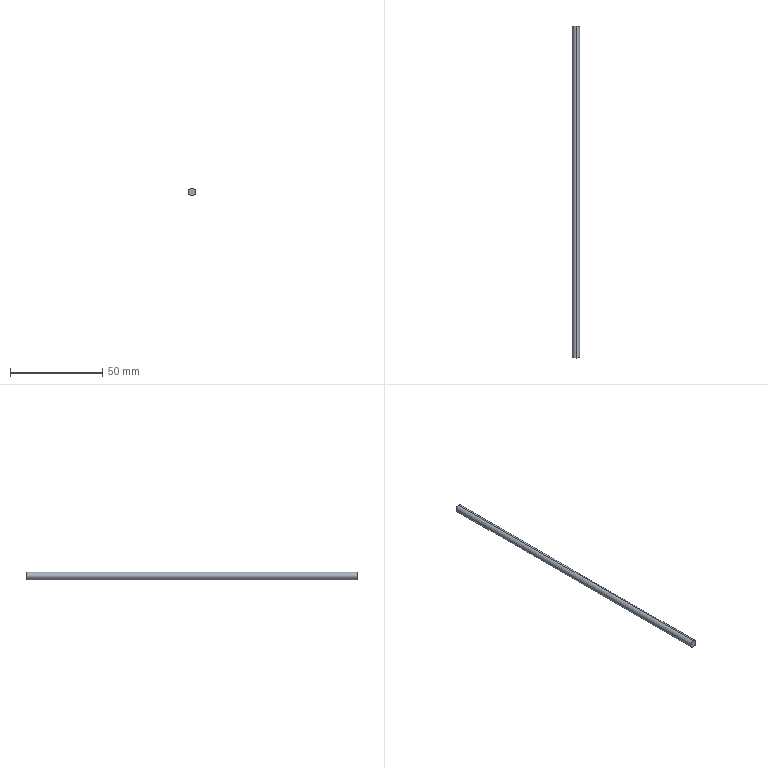Part | SolidWorks | features Extrusion 1 | 1 solid | 4 faces | box 4 x 180 x 4 mm | volume 2262 mm3 | cylinder 2 | plane 2 | commonest cylinder face diameters 4 x2
STEP:
#1=CARTESIAN_POINT('',(0.,180.,2.));
#2=VERTEX_POINT('',#1);
#3=CARTESIAN_POINT('',(0.,180.,-2.));
#4=VERTEX_POINT('',#3);
#5=CARTESIAN_POINT('',(0.,180.,0.));
#6=DIRECTION('',(0.,1.,0.));
#7=DIRECTION('',(0.,0.,1.));
#8=AXIS2_PLACEMENT_3D('',#5,#6,#7);
#9=CIRCLE('',#8,2.);
#10=EDGE_CURVE('',#2,#4,#9,.T.);
#11=ORIENTED_EDGE('',*,*,#10,.F.);
#12=CARTESIAN_POINT('',(0.,0.,2.));
#13=VERTEX_POINT('',#12);
#14=CARTESIAN_POINT('',(0.,180.,2.));
#15=DIRECTION('',(0.,-1.,0.));
#16=VECTOR('',#15,1000.);
#17=LINE('',#14,#16);
#18=EDGE_CURVE('',#2,#13,#17,.T.);
#19=ORIENTED_EDGE('',*,*,#18,.T.);
#20=CARTESIAN_POINT('',(0.,0.,-2.));
#21=VERTEX_POINT('',#20);
#22=CARTESIAN_POINT('',(0.,0.,0.));
#23=DIRECTION('',(0.,1.,0.));
#24=DIRECTION('',(0.,0.,1.));
#25=AXIS2_PLACEMENT_3D('',#22,#23,#24);
#26=CIRCLE('',#25,2.);
#27=EDGE_CURVE('',#13,#21,#26,.T.);
#28=ORIENTED_EDGE('',*,*,#27,.T.);
#29=CARTESIAN_POINT('',(0.,180.,-2.));
#30=DIRECTION('',(0.,-1.,0.));
#31=VECTOR('',#30,1000.);
#32=LINE('',#29,#31);
#33=EDGE_CURVE('',#4,#21,#32,.T.);
#34=ORIENTED_EDGE('',*,*,#33,.F.);
#35=EDGE_LOOP('',(#11,#19,#28,#34));
#36=FACE_OUTER_BOUND('',#35,.T.);
#37=CARTESIAN_POINT('',(0.,180.,0.));
#38=DIRECTION('',(0.,-1.,0.));
#39=DIRECTION('',(0.,0.,-1.));
#40=AXIS2_PLACEMENT_3D('',#37,#38,#39);
#41=CYLINDRICAL_SURFACE('',#40,2.);
#42=ADVANCED_FACE('',(#36),#41,.T.);
#43=ORIENTED_EDGE('',*,*,#18,.F.);
#44=CARTESIAN_POINT('',(0.,180.,0.));
#45=DIRECTION('',(0.,1.,0.));
#46=DIRECTION('',(0.,0.,1.));
#47=AXIS2_PLACEMENT_3D('',#44,#45,#46);
#48=CIRCLE('',#47,2.);
#49=EDGE_CURVE('',#4,#2,#48,.T.);
#50=ORIENTED_EDGE('',*,*,#49,.F.);
#51=ORIENTED_EDGE('',*,*,#33,.T.);
#52=CARTESIAN_POINT('',(0.,0.,0.));
#53=DIRECTION('',(0.,1.,0.));
#54=DIRECTION('',(0.,0.,1.));
#55=AXIS2_PLACEMENT_3D('',#52,#53,#54);
#56=CIRCLE('',#55,2.);
#57=EDGE_CURVE('',#21,#13,#56,.T.);
#58=ORIENTED_EDGE('',*,*,#57,.T.);
#59=EDGE_LOOP('',(#43,#50,#51,#58));
#60=FACE_OUTER_BOUND('',#59,.T.);
#61=CARTESIAN_POINT('',(0.,180.,0.));
#62=DIRECTION('',(0.,-1.,0.));
#63=DIRECTION('',(0.,0.,-1.));
#64=AXIS2_PLACEMENT_3D('',#61,#62,#63);
#65=CYLINDRICAL_SURFACE('',#64,2.);
#66=ADVANCED_FACE('',(#60),#65,.T.);
#67=ORIENTED_EDGE('',*,*,#49,.T.);
#68=ORIENTED_EDGE('',*,*,#10,.T.);
#69=EDGE_LOOP('',(#67,#68));
#70=FACE_OUTER_BOUND('',#69,.T.);
#71=CARTESIAN_POINT('',(0.,180.,0.));
#72=DIRECTION('',(0.,1.,0.));
#73=DIRECTION('',(0.,0.,1.));
#74=AXIS2_PLACEMENT_3D('',#71,#72,#73);
#75=PLANE('',#74);
#76=ADVANCED_FACE('',(#70),#75,.T.);
#77=ORIENTED_EDGE('',*,*,#57,.F.);
#78=ORIENTED_EDGE('',*,*,#27,.F.);
#79=EDGE_LOOP('',(#77,#78));
#80=FACE_OUTER_BOUND('',#79,.T.);
#81=CARTESIAN_POINT('',(0.,0.,0.));
#82=DIRECTION('',(0.,1.,0.));
#83=DIRECTION('',(0.,0.,1.));
#84=AXIS2_PLACEMENT_3D('',#81,#82,#83);
#85=PLANE('',#84);
#86=ADVANCED_FACE('',(#80),#85,.F.);
#87=CLOSED_SHELL('',(#42,#66,#76,#86));
#88=MANIFOLD_SOLID_BREP('',#87);
#89=CARTESIAN_POINT('',(0.,0.,0.));
#90=DIRECTION('',(0.,0.,1.));
#91=DIRECTION('',(1.,0.,0.));
#92=AXIS2_PLACEMENT_3D('',#89,#90,#91);
#93=(LENGTH_UNIT()NAMED_UNIT(*)SI_UNIT(.MILLI.,.METRE.));
#94=UNCERTAINTY_MEASURE_WITH_UNIT(LENGTH_MEASURE(0.00001),#93,'','');
#95=(NAMED_UNIT(*)PLANE_ANGLE_UNIT()SI_UNIT($,.RADIAN.));
#96=(NAMED_UNIT(*)SI_UNIT($,.STERADIAN.)SOLID_ANGLE_UNIT());
#97=(GEOMETRIC_REPRESENTATION_CONTEXT(3)GLOBAL_UNCERTAINTY_ASSIGNED_CONTEXT((#94))GLOBAL_UNIT_ASSIGNED_CONTEXT((#93,#95,#96))REPRESENTATION_CONTEXT('',''));
#98=ADVANCED_BREP_SHAPE_REPRESENTATION('',(#88,#92),#97);